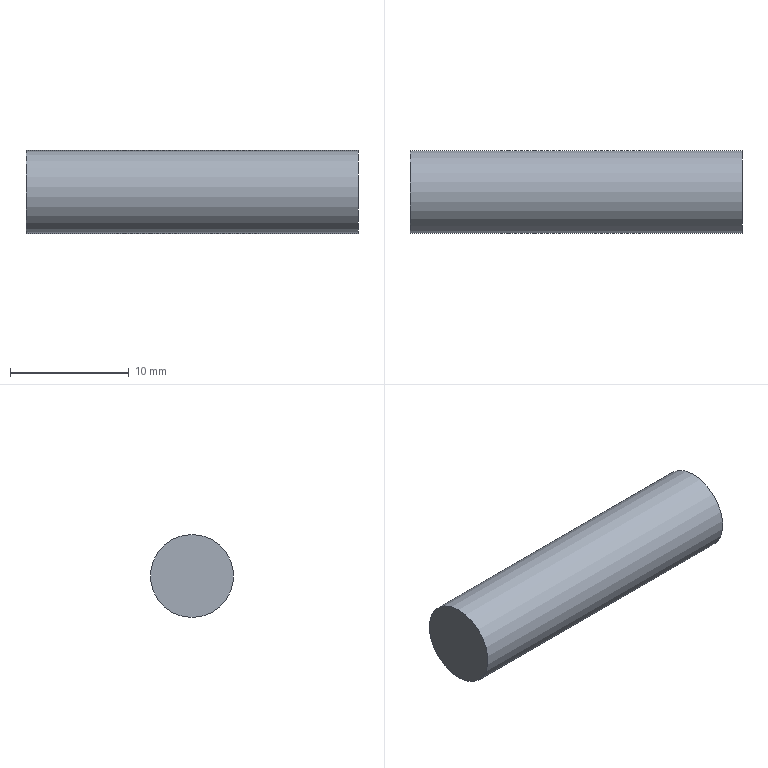Part | NX | features solid 2 | 1 solid | 3 faces | box 28 x 7 x 7 mm | volume 1078 mm3 | plane 2 | cylinder 1 | commonest cylinder face diameters 7 x1
STEP:
#1=CARTESIAN_POINT('',(-1554.,415.,12.5));
#2=VERTEX_POINT('',#1);
#3=CARTESIAN_POINT('',(-1554.,415.,16.));
#4=DIRECTION('',(1.,0.,0.));
#5=DIRECTION('',(0.,0.,-1.));
#6=AXIS2_PLACEMENT_3D('',#3,#4,#5);
#7=CIRCLE('',#6,3.5);
#8=EDGE_CURVE('',#2,#2,#7,.T.);
#9=ORIENTED_EDGE('',*,*,#8,.T.);
#10=EDGE_LOOP('',(#9));
#11=FACE_BOUND('',#10,.T.);
#12=CARTESIAN_POINT('',(-1526.,415.,12.5));
#13=VERTEX_POINT('',#12);
#14=CARTESIAN_POINT('',(-1526.,415.,16.));
#15=DIRECTION('',(1.,0.,0.));
#16=DIRECTION('',(0.,0.,-1.));
#17=AXIS2_PLACEMENT_3D('',#14,#15,#16);
#18=CIRCLE('',#17,3.5);
#19=EDGE_CURVE('',#13,#13,#18,.T.);
#20=ORIENTED_EDGE('',*,*,#19,.F.);
#21=EDGE_LOOP('',(#20));
#22=FACE_BOUND('',#21,.T.);
#23=CARTESIAN_POINT('',(-1554.,415.,16.));
#24=DIRECTION('',(1.,0.,0.));
#25=DIRECTION('',(0.,0.,-1.));
#26=AXIS2_PLACEMENT_3D('',#23,#24,#25);
#27=CYLINDRICAL_SURFACE('',#26,3.5);
#28=ADVANCED_FACE('',(#11,#22),#27,.T.);
#29=ORIENTED_EDGE('',*,*,#8,.F.);
#30=EDGE_LOOP('',(#29));
#31=FACE_BOUND('',#30,.T.);
#32=CARTESIAN_POINT('',(-1554.,415.,16.));
#33=DIRECTION('',(1.,0.,0.));
#34=DIRECTION('',(0.,0.,-1.));
#35=AXIS2_PLACEMENT_3D('',#32,#33,#34);
#36=PLANE('',#35);
#37=ADVANCED_FACE('',(#31),#36,.F.);
#38=ORIENTED_EDGE('',*,*,#19,.T.);
#39=EDGE_LOOP('',(#38));
#40=FACE_BOUND('',#39,.T.);
#41=CARTESIAN_POINT('',(-1526.,415.,16.));
#42=DIRECTION('',(1.,0.,0.));
#43=DIRECTION('',(0.,0.,-1.));
#44=AXIS2_PLACEMENT_3D('',#41,#42,#43);
#45=PLANE('',#44);
#46=ADVANCED_FACE('',(#40),#45,.T.);
#47=CLOSED_SHELL('',(#28,#37,#46));
#48=MANIFOLD_SOLID_BREP('',#47);
#49=(LENGTH_UNIT()NAMED_UNIT(*)SI_UNIT(.MILLI.,.METRE.));
#50=UNCERTAINTY_MEASURE_WITH_UNIT(LENGTH_MEASURE(0.00001),#49,'','');
#51=(NAMED_UNIT(*)PLANE_ANGLE_UNIT()SI_UNIT($,.RADIAN.));
#52=(NAMED_UNIT(*)SI_UNIT($,.STERADIAN.)SOLID_ANGLE_UNIT());
#53=(GEOMETRIC_REPRESENTATION_CONTEXT(3)GLOBAL_UNCERTAINTY_ASSIGNED_CONTEXT((#50))GLOBAL_UNIT_ASSIGNED_CONTEXT((#49,#51,#52))REPRESENTATION_CONTEXT('',''));
#54=ADVANCED_BREP_SHAPE_REPRESENTATION('',(#48),#53);